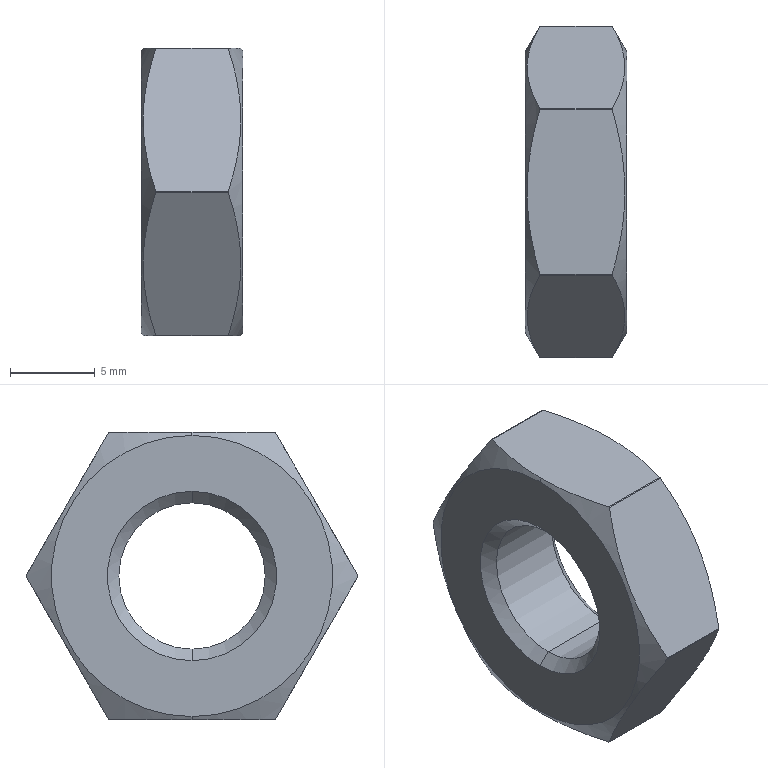Part | STEP file | Guide wheel mechanism revised.sldasm-Part-471 | 1 solid | 24 faces | box 6 x 19.6 x 17 mm | volume 1119 mm3 | cone 8 | cylinder 8 | plane 8 | commonest cylinder face diameters 19.6 x6 8.647 x2
STEP:
#1=CARTESIAN_POINT('',(5.324,0.,-4.324));
#2=VERTEX_POINT('',#1);
#3=CARTESIAN_POINT('',(5.324,0.,4.324));
#4=VERTEX_POINT('',#3);
#5=CARTESIAN_POINT('',(5.324,0.,0.));
#6=DIRECTION('',(-1.,0.,0.));
#7=DIRECTION('',(0.,0.,1.));
#8=AXIS2_PLACEMENT_3D('',#5,#6,#7);
#9=CIRCLE('',#8,4.324);
#10=EDGE_CURVE('',#2,#4,#9,.T.);
#11=ORIENTED_EDGE('',*,*,#10,.T.);
#12=CARTESIAN_POINT('',(6.,0.,5.));
#13=VERTEX_POINT('',#12);
#14=CARTESIAN_POINT('',(6.,0.,5.));
#15=DIRECTION('',(0.7071,0.,0.7071));
#16=VECTOR('',#15,1000.);
#17=LINE('',#14,#16);
#18=EDGE_CURVE('',#4,#13,#17,.T.);
#19=ORIENTED_EDGE('',*,*,#18,.T.);
#20=CARTESIAN_POINT('',(6.,0.,-5.));
#21=VERTEX_POINT('',#20);
#22=CARTESIAN_POINT('',(6.,0.,0.));
#23=DIRECTION('',(-1.,0.,0.));
#24=DIRECTION('',(0.,0.,1.));
#25=AXIS2_PLACEMENT_3D('',#22,#23,#24);
#26=CIRCLE('',#25,5.);
#27=EDGE_CURVE('',#21,#13,#26,.T.);
#28=ORIENTED_EDGE('',*,*,#27,.F.);
#29=CARTESIAN_POINT('',(6.,0.,-5.));
#30=DIRECTION('',(0.7071,0.,-0.7071));
#31=VECTOR('',#30,1000.);
#32=LINE('',#29,#31);
#33=EDGE_CURVE('',#2,#21,#32,.T.);
#34=ORIENTED_EDGE('',*,*,#33,.F.);
#35=EDGE_LOOP('',(#11,#19,#28,#34));
#36=FACE_OUTER_BOUND('',#35,.T.);
#37=CARTESIAN_POINT('',(6.,0.,0.));
#38=DIRECTION('',(1.,0.,0.));
#39=DIRECTION('',(0.,0.,-1.));
#40=AXIS2_PLACEMENT_3D('',#37,#38,#39);
#41=CONICAL_SURFACE('',#40,5.,0.7854);
#42=ADVANCED_FACE('',(#36),#41,.F.);
#43=ORIENTED_EDGE('',*,*,#10,.F.);
#44=CARTESIAN_POINT('',(0.6765,0.,-4.324));
#45=VERTEX_POINT('',#44);
#46=CARTESIAN_POINT('',(6.,0.,-4.324));
#47=DIRECTION('',(-1.,0.,0.));
#48=VECTOR('',#47,1000.);
#49=LINE('',#46,#48);
#50=EDGE_CURVE('',#2,#45,#49,.T.);
#51=ORIENTED_EDGE('',*,*,#50,.T.);
#52=CARTESIAN_POINT('',(0.6765,0.,4.324));
#53=VERTEX_POINT('',#52);
#54=CARTESIAN_POINT('',(0.6765,0.,0.));
#55=DIRECTION('',(-1.,0.,0.));
#56=DIRECTION('',(0.,0.,1.));
#57=AXIS2_PLACEMENT_3D('',#54,#55,#56);
#58=CIRCLE('',#57,4.324);
#59=EDGE_CURVE('',#45,#53,#58,.T.);
#60=ORIENTED_EDGE('',*,*,#59,.T.);
#61=CARTESIAN_POINT('',(6.,0.,4.324));
#62=DIRECTION('',(-1.,0.,0.));
#63=VECTOR('',#62,1000.);
#64=LINE('',#61,#63);
#65=EDGE_CURVE('',#4,#53,#64,.T.);
#66=ORIENTED_EDGE('',*,*,#65,.F.);
#67=EDGE_LOOP('',(#43,#51,#60,#66));
#68=FACE_OUTER_BOUND('',#67,.T.);
#69=CARTESIAN_POINT('',(6.,0.,0.));
#70=DIRECTION('',(-1.,0.,0.));
#71=DIRECTION('',(0.,0.,1.));
#72=AXIS2_PLACEMENT_3D('',#69,#70,#71);
#73=CYLINDRICAL_SURFACE('',#72,4.324);
#74=ADVANCED_FACE('',(#68),#73,.F.);
#75=ORIENTED_EDGE('',*,*,#59,.F.);
#76=CARTESIAN_POINT('',(0.,0.,-5.));
#77=VERTEX_POINT('',#76);
#78=CARTESIAN_POINT('',(0.6765,0.,-4.324));
#79=DIRECTION('',(-0.7071,0.,-0.7071));
#80=VECTOR('',#79,1000.);
#81=LINE('',#78,#80);
#82=EDGE_CURVE('',#45,#77,#81,.T.);
#83=ORIENTED_EDGE('',*,*,#82,.T.);
#84=CARTESIAN_POINT('',(0.,0.,5.));
#85=VERTEX_POINT('',#84);
#86=CARTESIAN_POINT('',(0.,0.,0.));
#87=DIRECTION('',(-1.,0.,0.));
#88=DIRECTION('',(0.,0.,1.));
#89=AXIS2_PLACEMENT_3D('',#86,#87,#88);
#90=CIRCLE('',#89,5.);
#91=EDGE_CURVE('',#77,#85,#90,.T.);
#92=ORIENTED_EDGE('',*,*,#91,.T.);
#93=CARTESIAN_POINT('',(0.6765,0.,4.324));
#94=DIRECTION('',(-0.7071,0.,0.7071));
#95=VECTOR('',#94,1000.);
#96=LINE('',#93,#95);
#97=EDGE_CURVE('',#53,#85,#96,.T.);
#98=ORIENTED_EDGE('',*,*,#97,.F.);
#99=EDGE_LOOP('',(#75,#83,#92,#98));
#100=FACE_OUTER_BOUND('',#99,.T.);
#101=CARTESIAN_POINT('',(0.6765,0.,0.));
#102=DIRECTION('',(-1.,0.,0.));
#103=DIRECTION('',(0.,0.,1.));
#104=AXIS2_PLACEMENT_3D('',#101,#102,#103);
#105=CONICAL_SURFACE('',#104,4.324,0.7854);
#106=ADVANCED_FACE('',(#100),#105,.F.);
#107=CARTESIAN_POINT('',(6.,0.,8.3));
#108=VERTEX_POINT('',#107);
#109=CARTESIAN_POINT('',(6.,0.,-8.3));
#110=VERTEX_POINT('',#109);
#111=CARTESIAN_POINT('',(6.,0.,0.));
#112=DIRECTION('',(-1.,0.,0.));
#113=DIRECTION('',(0.,0.,1.));
#114=AXIS2_PLACEMENT_3D('',#111,#112,#113);
#115=CIRCLE('',#114,8.3);
#116=EDGE_CURVE('',#108,#110,#115,.T.);
#117=ORIENTED_EDGE('',*,*,#116,.T.);
#118=CARTESIAN_POINT('',(5.885,0.,-8.5));
#119=VERTEX_POINT('',#118);
#120=CARTESIAN_POINT('',(6.,0.,-8.3));
#121=DIRECTION('',(-0.5,0.,-0.866));
#122=VECTOR('',#121,1000.);
#123=LINE('',#120,#122);
#124=EDGE_CURVE('',#110,#119,#123,.T.);
#125=ORIENTED_EDGE('',*,*,#124,.T.);
#126=CARTESIAN_POINT('',(5.134,4.877,-8.5));
#127=VERTEX_POINT('',#126);
#128=CARTESIAN_POINT('',(5.885,0.,-8.5));
#129=CARTESIAN_POINT('',(5.885,0.8245,-8.5));
#130=CARTESIAN_POINT('',(5.812,1.66,-8.5));
#131=CARTESIAN_POINT('',(5.549,3.29,-8.5));
#132=CARTESIAN_POINT('',(5.361,4.089,-8.5));
#133=CARTESIAN_POINT('',(5.134,4.877,-8.5));
#134=B_SPLINE_CURVE_WITH_KNOTS('',3,(#128,#129,#130,#131,#132,#133),.UNSPECIFIED.,.F.,.F.,(4,2,4),(0.0137,0.01617,0.01864),.UNSPECIFIED.);
#135=EDGE_CURVE('',#119,#127,#134,.T.);
#136=ORIENTED_EDGE('',*,*,#135,.T.);
#137=CARTESIAN_POINT('',(5.134,4.922,-8.474));
#138=VERTEX_POINT('',#137);
#139=CARTESIAN_POINT('',(5.134,0.,0.));
#140=DIRECTION('',(-1.,0.,0.));
#141=DIRECTION('',(0.,0.,1.));
#142=AXIS2_PLACEMENT_3D('',#139,#140,#141);
#143=CIRCLE('',#142,9.8);
#144=EDGE_CURVE('',#138,#127,#143,.T.);
#145=ORIENTED_EDGE('',*,*,#144,.F.);
#146=CARTESIAN_POINT('',(5.134,9.8,-0.02596));
#147=VERTEX_POINT('',#146);
#148=CARTESIAN_POINT('',(5.134,4.922,-8.474));
#149=CARTESIAN_POINT('',(5.363,5.321,-7.784));
#150=CARTESIAN_POINT('',(5.551,5.722,-7.089));
#151=CARTESIAN_POINT('',(5.812,6.532,-5.686));
#152=CARTESIAN_POINT('',(5.884,6.942,-4.976));
#153=CARTESIAN_POINT('',(5.885,7.564,-3.9));
#154=CARTESIAN_POINT('',(5.867,7.772,-3.539));
#155=CARTESIAN_POINT('',(5.799,8.184,-2.825));
#156=CARTESIAN_POINT('',(5.748,8.389,-2.47));
#157=CARTESIAN_POINT('',(5.552,8.999,-1.413));
#158=CARTESIAN_POINT('',(5.363,9.401,-0.7167));
#159=CARTESIAN_POINT('',(5.134,9.8,-0.02596));
#160=B_SPLINE_CURVE_WITH_KNOTS('',3,(#148,#149,#150,#151,#152,#153,#154,#155,#156,#157,#158,#159),.UNSPECIFIED.,.F.,.F.,(4,2,2,2,2,4),(0.000000717,0.002463,0.004926,0.006157,0.007388,0.00985),.UNSPECIFIED.);
#161=EDGE_CURVE('',#138,#147,#160,.T.);
#162=ORIENTED_EDGE('',*,*,#161,.T.);
#163=CARTESIAN_POINT('',(5.134,9.8,0.02596));
#164=VERTEX_POINT('',#163);
#165=CARTESIAN_POINT('',(5.134,0.,0.));
#166=DIRECTION('',(-1.,0.,0.));
#167=DIRECTION('',(0.,0.,1.));
#168=AXIS2_PLACEMENT_3D('',#165,#166,#167);
#169=CIRCLE('',#168,9.8);
#170=EDGE_CURVE('',#164,#147,#169,.T.);
#171=ORIENTED_EDGE('',*,*,#170,.F.);
#172=CARTESIAN_POINT('',(5.134,4.922,8.474));
#173=VERTEX_POINT('',#172);
#174=CARTESIAN_POINT('',(5.134,9.8,0.02596));
#175=CARTESIAN_POINT('',(5.363,9.402,0.7158));
#176=CARTESIAN_POINT('',(5.551,9.001,1.411));
#177=CARTESIAN_POINT('',(5.812,8.19,2.814));
#178=CARTESIAN_POINT('',(5.884,7.781,3.524));
#179=CARTESIAN_POINT('',(5.885,7.159,4.6));
#180=CARTESIAN_POINT('',(5.867,6.951,4.961));
#181=CARTESIAN_POINT('',(5.799,6.538,5.675));
#182=CARTESIAN_POINT('',(5.748,6.334,6.03));
#183=CARTESIAN_POINT('',(5.552,5.723,7.087));
#184=CARTESIAN_POINT('',(5.363,5.321,7.783));
#185=CARTESIAN_POINT('',(5.134,4.922,8.474));
#186=B_SPLINE_CURVE_WITH_KNOTS('',3,(#174,#175,#176,#177,#178,#179,#180,#181,#182,#183,#184,#185),.UNSPECIFIED.,.F.,.F.,(4,2,2,2,2,4),(0.000000483,0.002463,0.004925,0.006157,0.007388,0.00985),.UNSPECIFIED.);
#187=EDGE_CURVE('',#164,#173,#186,.T.);
#188=ORIENTED_EDGE('',*,*,#187,.T.);
#189=CARTESIAN_POINT('',(5.134,4.877,8.5));
#190=VERTEX_POINT('',#189);
#191=CARTESIAN_POINT('',(5.134,0.,0.));
#192=DIRECTION('',(-1.,0.,0.));
#193=DIRECTION('',(0.,0.,1.));
#194=AXIS2_PLACEMENT_3D('',#191,#192,#193);
#195=CIRCLE('',#194,9.8);
#196=EDGE_CURVE('',#190,#173,#195,.T.);
#197=ORIENTED_EDGE('',*,*,#196,.F.);
#198=CARTESIAN_POINT('',(5.885,0.,8.5));
#199=VERTEX_POINT('',#198);
#200=CARTESIAN_POINT('',(5.134,4.877,8.5));
#201=CARTESIAN_POINT('',(5.361,4.089,8.5));
#202=CARTESIAN_POINT('',(5.549,3.29,8.5));
#203=CARTESIAN_POINT('',(5.812,1.66,8.5));
#204=CARTESIAN_POINT('',(5.885,0.8245,8.5));
#205=CARTESIAN_POINT('',(5.885,0.,8.5));
#206=B_SPLINE_CURVE_WITH_KNOTS('',3,(#200,#201,#202,#203,#204,#205),.UNSPECIFIED.,.F.,.F.,(4,2,4),(0.003649,0.006111,0.008573),.UNSPECIFIED.);
#207=EDGE_CURVE('',#190,#199,#206,.T.);
#208=ORIENTED_EDGE('',*,*,#207,.T.);
#209=CARTESIAN_POINT('',(6.,0.,8.3));
#210=DIRECTION('',(-0.5,0.,0.866));
#211=VECTOR('',#210,1000.);
#212=LINE('',#209,#211);
#213=EDGE_CURVE('',#108,#199,#212,.T.);
#214=ORIENTED_EDGE('',*,*,#213,.F.);
#215=EDGE_LOOP('',(#117,#125,#136,#145,#162,#171,#188,#197,#208,#214));
#216=FACE_OUTER_BOUND('',#215,.T.);
#217=CARTESIAN_POINT('',(6.,0.,0.));
#218=DIRECTION('',(-1.,0.,0.));
#219=DIRECTION('',(0.,0.,1.));
#220=AXIS2_PLACEMENT_3D('',#217,#218,#219);
#221=CONICAL_SURFACE('',#220,8.3,1.047);
#222=ADVANCED_FACE('',(#216),#221,.T.);
#223=CARTESIAN_POINT('',(0.,0.,8.3));
#224=VERTEX_POINT('',#223);
#225=CARTESIAN_POINT('',(0.,0.,-8.3));
#226=VERTEX_POINT('',#225);
#227=CARTESIAN_POINT('',(0.,0.,0.));
#228=DIRECTION('',(-1.,0.,0.));
#229=DIRECTION('',(0.,0.,1.));
#230=AXIS2_PLACEMENT_3D('',#227,#228,#229);
#231=CIRCLE('',#230,8.3);
#232=EDGE_CURVE('',#224,#226,#231,.T.);
#233=ORIENTED_EDGE('',*,*,#232,.F.);
#234=CARTESIAN_POINT('',(0.1155,0.,8.5));
#235=VERTEX_POINT('',#234);
#236=CARTESIAN_POINT('',(0.866,0.,9.8));
#237=DIRECTION('',(0.5,0.,0.866));
#238=VECTOR('',#237,1000.);
#239=LINE('',#236,#238);
#240=EDGE_CURVE('',#224,#235,#239,.T.);
#241=ORIENTED_EDGE('',*,*,#240,.T.);
#242=CARTESIAN_POINT('',(0.866,4.877,8.5));
#243=VERTEX_POINT('',#242);
#244=CARTESIAN_POINT('',(0.1155,0.,8.5));
#245=CARTESIAN_POINT('',(0.1155,0.8245,8.5));
#246=CARTESIAN_POINT('',(0.1878,1.66,8.5));
#247=CARTESIAN_POINT('',(0.4508,3.29,8.5));
#248=CARTESIAN_POINT('',(0.6394,4.089,8.5));
#249=CARTESIAN_POINT('',(0.866,4.877,8.5));
#250=B_SPLINE_CURVE_WITH_KNOTS('',3,(#244,#245,#246,#247,#248,#249),.UNSPECIFIED.,.F.,.F.,(4,2,4),(0.0137,0.01617,0.01864),.UNSPECIFIED.);
#251=EDGE_CURVE('',#235,#243,#250,.T.);
#252=ORIENTED_EDGE('',*,*,#251,.T.);
#253=CARTESIAN_POINT('',(0.866,4.922,8.474));
#254=VERTEX_POINT('',#253);
#255=CARTESIAN_POINT('',(0.866,0.,0.));
#256=DIRECTION('',(-1.,0.,0.));
#257=DIRECTION('',(0.,0.,1.));
#258=AXIS2_PLACEMENT_3D('',#255,#256,#257);
#259=CIRCLE('',#258,9.8);
#260=EDGE_CURVE('',#243,#254,#259,.T.);
#261=ORIENTED_EDGE('',*,*,#260,.T.);
#262=CARTESIAN_POINT('',(0.866,9.8,0.02596));
#263=VERTEX_POINT('',#262);
#264=CARTESIAN_POINT('',(0.866,4.922,8.474));
#265=CARTESIAN_POINT('',(0.6371,5.321,7.784));
#266=CARTESIAN_POINT('',(0.4487,5.722,7.089));
#267=CARTESIAN_POINT('',(0.1877,6.532,5.686));
#268=CARTESIAN_POINT('',(0.116,6.942,4.976));
#269=CARTESIAN_POINT('',(0.1152,7.564,3.9));
#270=CARTESIAN_POINT('',(0.1327,7.772,3.539));
#271=CARTESIAN_POINT('',(0.201,8.184,2.825));
#272=CARTESIAN_POINT('',(0.2518,8.389,2.47));
#273=CARTESIAN_POINT('',(0.4479,8.999,1.413));
#274=CARTESIAN_POINT('',(0.6368,9.401,0.7167));
#275=CARTESIAN_POINT('',(0.866,9.8,0.02596));
#276=B_SPLINE_CURVE_WITH_KNOTS('',3,(#264,#265,#266,#267,#268,#269,#270,#271,#272,#273,#274,#275),.UNSPECIFIED.,.F.,.F.,(4,2,2,2,2,4),(0.000000717,0.002463,0.004926,0.006157,0.007388,0.00985),.UNSPECIFIED.);
#277=EDGE_CURVE('',#254,#263,#276,.T.);
#278=ORIENTED_EDGE('',*,*,#277,.T.);
#279=CARTESIAN_POINT('',(0.866,9.8,-0.02596));
#280=VERTEX_POINT('',#279);
#281=CARTESIAN_POINT('',(0.866,0.,0.));
#282=DIRECTION('',(-1.,0.,0.));
#283=DIRECTION('',(0.,0.,1.));
#284=AXIS2_PLACEMENT_3D('',#281,#282,#283);
#285=CIRCLE('',#284,9.8);
#286=EDGE_CURVE('',#263,#280,#285,.T.);
#287=ORIENTED_EDGE('',*,*,#286,.T.);
#288=CARTESIAN_POINT('',(0.866,4.922,-8.474));
#289=VERTEX_POINT('',#288);
#290=CARTESIAN_POINT('',(0.866,9.8,-0.02596));
#291=CARTESIAN_POINT('',(0.6371,9.402,-0.7158));
#292=CARTESIAN_POINT('',(0.4487,9.001,-1.411));
#293=CARTESIAN_POINT('',(0.1877,8.19,-2.814));
#294=CARTESIAN_POINT('',(0.116,7.781,-3.524));
#295=CARTESIAN_POINT('',(0.1152,7.159,-4.6));
#296=CARTESIAN_POINT('',(0.1327,6.951,-4.961));
#297=CARTESIAN_POINT('',(0.201,6.538,-5.675));
#298=CARTESIAN_POINT('',(0.2518,6.334,-6.03));
#299=CARTESIAN_POINT('',(0.4479,5.723,-7.087));
#300=CARTESIAN_POINT('',(0.6368,5.321,-7.783));
#301=CARTESIAN_POINT('',(0.866,4.922,-8.474));
#302=B_SPLINE_CURVE_WITH_KNOTS('',3,(#290,#291,#292,#293,#294,#295,#296,#297,#298,#299,#300,#301),.UNSPECIFIED.,.F.,.F.,(4,2,2,2,2,4),(0.000000483,0.002463,0.004925,0.006157,0.007388,0.00985),.UNSPECIFIED.);
#303=EDGE_CURVE('',#280,#289,#302,.T.);
#304=ORIENTED_EDGE('',*,*,#303,.T.);
#305=CARTESIAN_POINT('',(0.866,4.877,-8.5));
#306=VERTEX_POINT('',#305);
#307=CARTESIAN_POINT('',(0.866,0.,0.));
#308=DIRECTION('',(-1.,0.,0.));
#309=DIRECTION('',(0.,0.,1.));
#310=AXIS2_PLACEMENT_3D('',#307,#308,#309);
#311=CIRCLE('',#310,9.8);
#312=EDGE_CURVE('',#289,#306,#311,.T.);
#313=ORIENTED_EDGE('',*,*,#312,.T.);
#314=CARTESIAN_POINT('',(0.1155,0.,-8.5));
#315=VERTEX_POINT('',#314);
#316=CARTESIAN_POINT('',(0.866,4.877,-8.5));
#317=CARTESIAN_POINT('',(0.6394,4.089,-8.5));
#318=CARTESIAN_POINT('',(0.4508,3.29,-8.5));
#319=CARTESIAN_POINT('',(0.1878,1.66,-8.5));
#320=CARTESIAN_POINT('',(0.1155,0.8245,-8.5));
#321=CARTESIAN_POINT('',(0.1155,0.,-8.5));
#322=B_SPLINE_CURVE_WITH_KNOTS('',3,(#316,#317,#318,#319,#320,#321),.UNSPECIFIED.,.F.,.F.,(4,2,4),(0.003649,0.006111,0.008573),.UNSPECIFIED.);
#323=EDGE_CURVE('',#306,#315,#322,.T.);
#324=ORIENTED_EDGE('',*,*,#323,.T.);
#325=CARTESIAN_POINT('',(0.866,0.,-9.8));
#326=DIRECTION('',(0.5,0.,-0.866));
#327=VECTOR('',#326,1000.);
#328=LINE('',#325,#327);
#329=EDGE_CURVE('',#226,#315,#328,.T.);
#330=ORIENTED_EDGE('',*,*,#329,.F.);
#331=EDGE_LOOP('',(#233,#241,#252,#261,#278,#287,#304,#313,#324,#330));
#332=FACE_OUTER_BOUND('',#331,.T.);
#333=CARTESIAN_POINT('',(0.866,0.,0.));
#334=DIRECTION('',(1.,0.,0.));
#335=DIRECTION('',(0.,0.,-1.));
#336=AXIS2_PLACEMENT_3D('',#333,#334,#335);
#337=CONICAL_SURFACE('',#336,9.8,1.047);
#338=ADVANCED_FACE('',(#332),#337,.T.);
#339=CARTESIAN_POINT('',(0.,0.,0.));
#340=DIRECTION('',(-1.,0.,0.));
#341=DIRECTION('',(0.,0.,1.));
#342=AXIS2_PLACEMENT_3D('',#339,#340,#341);
#343=CIRCLE('',#342,8.3);
#344=EDGE_CURVE('',#226,#224,#343,.T.);
#345=ORIENTED_EDGE('',*,*,#344,.T.);
#346=ORIENTED_EDGE('',*,*,#232,.T.);
#347=EDGE_LOOP('',(#345,#346));
#348=FACE_OUTER_BOUND('',#347,.T.);
#349=CARTESIAN_POINT('',(0.,0.,0.));
#350=DIRECTION('',(-1.,0.,0.));
#351=DIRECTION('',(0.,0.,1.));
#352=AXIS2_PLACEMENT_3D('',#349,#350,#351);
#353=CIRCLE('',#352,5.);
#354=EDGE_CURVE('',#85,#77,#353,.T.);
#355=ORIENTED_EDGE('',*,*,#354,.F.);
#356=ORIENTED_EDGE('',*,*,#91,.F.);
#357=EDGE_LOOP('',(#355,#356));
#358=FACE_BOUND('',#357,.T.);
#359=CARTESIAN_POINT('',(0.,0.,0.));
#360=DIRECTION('',(1.,0.,0.));
#361=DIRECTION('',(0.,0.,-1.));
#362=AXIS2_PLACEMENT_3D('',#359,#360,#361);
#363=PLANE('',#362);
#364=ADVANCED_FACE('',(#348,#358),#363,.F.);
#365=ORIENTED_EDGE('',*,*,#116,.F.);
#366=CARTESIAN_POINT('',(6.,0.,0.));
#367=DIRECTION('',(-1.,0.,0.));
#368=DIRECTION('',(0.,0.,1.));
#369=AXIS2_PLACEMENT_3D('',#366,#367,#368);
#370=CIRCLE('',#369,8.3);
#371=EDGE_CURVE('',#110,#108,#370,.T.);
#372=ORIENTED_EDGE('',*,*,#371,.F.);
#373=EDGE_LOOP('',(#365,#372));
#374=FACE_OUTER_BOUND('',#373,.T.);
#375=ORIENTED_EDGE('',*,*,#27,.T.);
#376=CARTESIAN_POINT('',(6.,0.,0.));
#377=DIRECTION('',(-1.,0.,0.));
#378=DIRECTION('',(0.,0.,1.));
#379=AXIS2_PLACEMENT_3D('',#376,#377,#378);
#380=CIRCLE('',#379,5.);
#381=EDGE_CURVE('',#13,#21,#380,.T.);
#382=ORIENTED_EDGE('',*,*,#381,.T.);
#383=EDGE_LOOP('',(#375,#382));
#384=FACE_BOUND('',#383,.T.);
#385=CARTESIAN_POINT('',(6.,8.3,0.));
#386=DIRECTION('',(-1.,0.,0.));
#387=DIRECTION('',(0.,0.,1.));
#388=AXIS2_PLACEMENT_3D('',#385,#386,#387);
#389=PLANE('',#388);
#390=ADVANCED_FACE('',(#374,#384),#389,.F.);
#391=ORIENTED_EDGE('',*,*,#196,.T.);
#392=CARTESIAN_POINT('',(6.,4.922,8.474));
#393=DIRECTION('',(-1.,0.,0.));
#394=VECTOR('',#393,1000.);
#395=LINE('',#392,#394);
#396=EDGE_CURVE('',#173,#254,#395,.T.);
#397=ORIENTED_EDGE('',*,*,#396,.T.);
#398=ORIENTED_EDGE('',*,*,#260,.F.);
#399=CARTESIAN_POINT('',(6.,4.877,8.5));
#400=DIRECTION('',(1.,0.,0.));
#401=VECTOR('',#400,1000.);
#402=LINE('',#399,#401);
#403=EDGE_CURVE('',#243,#190,#402,.T.);
#404=ORIENTED_EDGE('',*,*,#403,.T.);
#405=EDGE_LOOP('',(#391,#397,#398,#404));
#406=FACE_OUTER_BOUND('',#405,.T.);
#407=CARTESIAN_POINT('',(6.,0.,0.));
#408=DIRECTION('',(-1.,0.,0.));
#409=DIRECTION('',(0.,0.,1.));
#410=AXIS2_PLACEMENT_3D('',#407,#408,#409);
#411=CYLINDRICAL_SURFACE('',#410,9.8);
#412=ADVANCED_FACE('',(#406),#411,.T.);
#413=CARTESIAN_POINT('',(5.134,-4.922,8.474));
#414=VERTEX_POINT('',#413);
#415=CARTESIAN_POINT('',(5.134,-4.877,8.5));
#416=VERTEX_POINT('',#415);
#417=CARTESIAN_POINT('',(5.134,0.,0.));
#418=DIRECTION('',(-1.,0.,0.));
#419=DIRECTION('',(0.,0.,1.));
#420=AXIS2_PLACEMENT_3D('',#417,#418,#419);
#421=CIRCLE('',#420,9.8);
#422=EDGE_CURVE('',#414,#416,#421,.T.);
#423=ORIENTED_EDGE('',*,*,#422,.T.);
#424=CARTESIAN_POINT('',(0.866,-4.877,8.5));
#425=VERTEX_POINT('',#424);
#426=CARTESIAN_POINT('',(6.,-4.877,8.5));
#427=DIRECTION('',(-1.,0.,0.));
#428=VECTOR('',#427,1000.);
#429=LINE('',#426,#428);
#430=EDGE_CURVE('',#416,#425,#429,.T.);
#431=ORIENTED_EDGE('',*,*,#430,.T.);
#432=CARTESIAN_POINT('',(0.866,-4.922,8.474));
#433=VERTEX_POINT('',#432);
#434=CARTESIAN_POINT('',(0.866,0.,0.));
#435=DIRECTION('',(-1.,0.,0.));
#436=DIRECTION('',(0.,0.,1.));
#437=AXIS2_PLACEMENT_3D('',#434,#435,#436);
#438=CIRCLE('',#437,9.8);
#439=EDGE_CURVE('',#433,#425,#438,.T.);
#440=ORIENTED_EDGE('',*,*,#439,.F.);
#441=CARTESIAN_POINT('',(6.,-4.922,8.474));
#442=DIRECTION('',(1.,0.,0.));
#443=VECTOR('',#442,1000.);
#444=LINE('',#441,#443);
#445=EDGE_CURVE('',#433,#414,#444,.T.);
#446=ORIENTED_EDGE('',*,*,#445,.T.);
#447=EDGE_LOOP('',(#423,#431,#440,#446));
#448=FACE_OUTER_BOUND('',#447,.T.);
#449=CARTESIAN_POINT('',(6.,0.,0.));
#450=DIRECTION('',(-1.,0.,0.));
#451=DIRECTION('',(0.,0.,1.));
#452=AXIS2_PLACEMENT_3D('',#449,#450,#451);
#453=CYLINDRICAL_SURFACE('',#452,9.8);
#454=ADVANCED_FACE('',(#448),#453,.T.);
#455=CARTESIAN_POINT('',(5.134,-9.8,-0.02596));
#456=VERTEX_POINT('',#455);
#457=CARTESIAN_POINT('',(5.134,-9.8,0.02596));
#458=VERTEX_POINT('',#457);
#459=CARTESIAN_POINT('',(5.134,0.,0.));
#460=DIRECTION('',(-1.,0.,0.));
#461=DIRECTION('',(0.,0.,1.));
#462=AXIS2_PLACEMENT_3D('',#459,#460,#461);
#463=CIRCLE('',#462,9.8);
#464=EDGE_CURVE('',#456,#458,#463,.T.);
#465=ORIENTED_EDGE('',*,*,#464,.T.);
#466=CARTESIAN_POINT('',(0.866,-9.8,0.02596));
#467=VERTEX_POINT('',#466);
#468=CARTESIAN_POINT('',(6.,-9.8,0.02596));
#469=DIRECTION('',(-1.,0.,0.));
#470=VECTOR('',#469,1000.);
#471=LINE('',#468,#470);
#472=EDGE_CURVE('',#458,#467,#471,.T.);
#473=ORIENTED_EDGE('',*,*,#472,.T.);
#474=CARTESIAN_POINT('',(0.866,-9.8,-0.02596));
#475=VERTEX_POINT('',#474);
#476=CARTESIAN_POINT('',(0.866,0.,0.));
#477=DIRECTION('',(-1.,0.,0.));
#478=DIRECTION('',(0.,0.,1.));
#479=AXIS2_PLACEMENT_3D('',#476,#477,#478);
#480=CIRCLE('',#479,9.8);
#481=EDGE_CURVE('',#475,#467,#480,.T.);
#482=ORIENTED_EDGE('',*,*,#481,.F.);
#483=CARTESIAN_POINT('',(6.,-9.8,-0.02596));
#484=DIRECTION('',(1.,0.,0.));
#485=VECTOR('',#484,1000.);
#486=LINE('',#483,#485);
#487=EDGE_CURVE('',#475,#456,#486,.T.);
#488=ORIENTED_EDGE('',*,*,#487,.T.);
#489=EDGE_LOOP('',(#465,#473,#482,#488));
#490=FACE_OUTER_BOUND('',#489,.T.);
#491=CARTESIAN_POINT('',(6.,0.,0.));
#492=DIRECTION('',(-1.,0.,0.));
#493=DIRECTION('',(0.,0.,1.));
#494=AXIS2_PLACEMENT_3D('',#491,#492,#493);
#495=CYLINDRICAL_SURFACE('',#494,9.8);
#496=ADVANCED_FACE('',(#490),#495,.T.);
#497=CARTESIAN_POINT('',(5.134,-4.877,-8.5));
#498=VERTEX_POINT('',#497);
#499=CARTESIAN_POINT('',(5.134,-4.922,-8.474));
#500=VERTEX_POINT('',#499);
#501=CARTESIAN_POINT('',(5.134,0.,0.));
#502=DIRECTION('',(-1.,0.,0.));
#503=DIRECTION('',(0.,0.,1.));
#504=AXIS2_PLACEMENT_3D('',#501,#502,#503);
#505=CIRCLE('',#504,9.8);
#506=EDGE_CURVE('',#498,#500,#505,.T.);
#507=ORIENTED_EDGE('',*,*,#506,.T.);
#508=CARTESIAN_POINT('',(0.866,-4.922,-8.474));
#509=VERTEX_POINT('',#508);
#510=CARTESIAN_POINT('',(6.,-4.922,-8.474));
#511=DIRECTION('',(-1.,0.,0.));
#512=VECTOR('',#511,1000.);
#513=LINE('',#510,#512);
#514=EDGE_CURVE('',#500,#509,#513,.T.);
#515=ORIENTED_EDGE('',*,*,#514,.T.);
#516=CARTESIAN_POINT('',(0.866,-4.877,-8.5));
#517=VERTEX_POINT('',#516);
#518=CARTESIAN_POINT('',(0.866,0.,0.));
#519=DIRECTION('',(-1.,0.,0.));
#520=DIRECTION('',(0.,0.,1.));
#521=AXIS2_PLACEMENT_3D('',#518,#519,#520);
#522=CIRCLE('',#521,9.8);
#523=EDGE_CURVE('',#517,#509,#522,.T.);
#524=ORIENTED_EDGE('',*,*,#523,.F.);
#525=CARTESIAN_POINT('',(6.,-4.877,-8.5));
#526=DIRECTION('',(1.,0.,0.));
#527=VECTOR('',#526,1000.);
#528=LINE('',#525,#527);
#529=EDGE_CURVE('',#517,#498,#528,.T.);
#530=ORIENTED_EDGE('',*,*,#529,.T.);
#531=EDGE_LOOP('',(#507,#515,#524,#530));
#532=FACE_OUTER_BOUND('',#531,.T.);
#533=CARTESIAN_POINT('',(6.,0.,0.));
#534=DIRECTION('',(-1.,0.,0.));
#535=DIRECTION('',(0.,0.,1.));
#536=AXIS2_PLACEMENT_3D('',#533,#534,#535);
#537=CYLINDRICAL_SURFACE('',#536,9.8);
#538=ADVANCED_FACE('',(#532),#537,.T.);
#539=ORIENTED_EDGE('',*,*,#144,.T.);
#540=CARTESIAN_POINT('',(6.,4.877,-8.5));
#541=DIRECTION('',(-1.,0.,0.));
#542=VECTOR('',#541,1000.);
#543=LINE('',#540,#542);
#544=EDGE_CURVE('',#127,#306,#543,.T.);
#545=ORIENTED_EDGE('',*,*,#544,.T.);
#546=ORIENTED_EDGE('',*,*,#312,.F.);
#547=CARTESIAN_POINT('',(6.,4.922,-8.474));
#548=DIRECTION('',(1.,0.,0.));
#549=VECTOR('',#548,1000.);
#550=LINE('',#547,#549);
#551=EDGE_CURVE('',#289,#138,#550,.T.);
#552=ORIENTED_EDGE('',*,*,#551,.T.);
#553=EDGE_LOOP('',(#539,#545,#546,#552));
#554=FACE_OUTER_BOUND('',#553,.T.);
#555=CARTESIAN_POINT('',(6.,0.,0.));
#556=DIRECTION('',(-1.,0.,0.));
#557=DIRECTION('',(0.,0.,1.));
#558=AXIS2_PLACEMENT_3D('',#555,#556,#557);
#559=CYLINDRICAL_SURFACE('',#558,9.8);
#560=ADVANCED_FACE('',(#554),#559,.T.);
#561=ORIENTED_EDGE('',*,*,#240,.F.);
#562=ORIENTED_EDGE('',*,*,#344,.F.);
#563=ORIENTED_EDGE('',*,*,#329,.T.);
#564=CARTESIAN_POINT('',(0.1155,0.,-8.5));
#565=CARTESIAN_POINT('',(0.1155,-0.824,-8.5));
#566=CARTESIAN_POINT('',(0.1858,-1.643,-8.5));
#567=CARTESIAN_POINT('',(0.447,-3.271,-8.5));
#568=CARTESIAN_POINT('',(0.638,-4.084,-8.5));
#569=CARTESIAN_POINT('',(0.866,-4.877,-8.5));
#570=B_SPLINE_CURVE_WITH_KNOTS('',3,(#564,#565,#566,#567,#568,#569),.UNSPECIFIED.,.F.,.F.,(4,2,4),(0.008573,0.01103,0.01349),.UNSPECIFIED.);
#571=EDGE_CURVE('',#315,#517,#570,.T.);
#572=ORIENTED_EDGE('',*,*,#571,.T.);
#573=ORIENTED_EDGE('',*,*,#523,.T.);
#574=CARTESIAN_POINT('',(0.866,-4.922,-8.474));
#575=CARTESIAN_POINT('',(0.6371,-5.321,-7.784));
#576=CARTESIAN_POINT('',(0.4487,-5.722,-7.089));
#577=CARTESIAN_POINT('',(0.1877,-6.532,-5.686));
#578=CARTESIAN_POINT('',(0.116,-6.942,-4.976));
#579=CARTESIAN_POINT('',(0.1152,-7.564,-3.9));
#580=CARTESIAN_POINT('',(0.1327,-7.772,-3.539));
#581=CARTESIAN_POINT('',(0.201,-8.184,-2.825));
#582=CARTESIAN_POINT('',(0.2518,-8.389,-2.47));
#583=CARTESIAN_POINT('',(0.4479,-8.999,-1.413));
#584=CARTESIAN_POINT('',(0.6368,-9.401,-0.7167));
#585=CARTESIAN_POINT('',(0.866,-9.8,-0.02596));
#586=B_SPLINE_CURVE_WITH_KNOTS('',3,(#574,#575,#576,#577,#578,#579,#580,#581,#582,#583,#584,#585),.UNSPECIFIED.,.F.,.F.,(4,2,2,2,2,4),(0.000000717,0.002463,0.004926,0.006157,0.007388,0.00985),.UNSPECIFIED.);
#587=EDGE_CURVE('',#509,#475,#586,.T.);
#588=ORIENTED_EDGE('',*,*,#587,.T.);
#589=ORIENTED_EDGE('',*,*,#481,.T.);
#590=CARTESIAN_POINT('',(0.866,-9.8,0.02596));
#591=CARTESIAN_POINT('',(0.6371,-9.402,0.7158));
#592=CARTESIAN_POINT('',(0.4487,-9.001,1.411));
#593=CARTESIAN_POINT('',(0.1877,-8.19,2.814));
#594=CARTESIAN_POINT('',(0.116,-7.781,3.524));
#595=CARTESIAN_POINT('',(0.1152,-7.159,4.6));
#596=CARTESIAN_POINT('',(0.1327,-6.951,4.961));
#597=CARTESIAN_POINT('',(0.201,-6.538,5.675));
#598=CARTESIAN_POINT('',(0.2518,-6.334,6.03));
#599=CARTESIAN_POINT('',(0.4479,-5.723,7.087));
#600=CARTESIAN_POINT('',(0.6368,-5.321,7.783));
#601=CARTESIAN_POINT('',(0.866,-4.922,8.474));
#602=B_SPLINE_CURVE_WITH_KNOTS('',3,(#590,#591,#592,#593,#594,#595,#596,#597,#598,#599,#600,#601),.UNSPECIFIED.,.F.,.F.,(4,2,2,2,2,4),(0.000000483,0.002463,0.004925,0.006157,0.007388,0.00985),.UNSPECIFIED.);
#603=EDGE_CURVE('',#467,#433,#602,.T.);
#604=ORIENTED_EDGE('',*,*,#603,.T.);
#605=ORIENTED_EDGE('',*,*,#439,.T.);
#606=CARTESIAN_POINT('',(0.866,-4.877,8.5));
#607=CARTESIAN_POINT('',(0.638,-4.084,8.5));
#608=CARTESIAN_POINT('',(0.447,-3.271,8.5));
#609=CARTESIAN_POINT('',(0.1858,-1.643,8.5));
#610=CARTESIAN_POINT('',(0.1155,-0.824,8.5));
#611=CARTESIAN_POINT('',(0.1155,0.,8.5));
#612=B_SPLINE_CURVE_WITH_KNOTS('',3,(#606,#607,#608,#609,#610,#611),.UNSPECIFIED.,.F.,.F.,(4,2,4),(0.008768,0.01123,0.0137),.UNSPECIFIED.);
#613=EDGE_CURVE('',#425,#235,#612,.T.);
#614=ORIENTED_EDGE('',*,*,#613,.T.);
#615=EDGE_LOOP('',(#561,#562,#563,#572,#573,#588,#589,#604,#605,#614));
#616=FACE_OUTER_BOUND('',#615,.T.);
#617=CARTESIAN_POINT('',(0.866,0.,0.));
#618=DIRECTION('',(1.,0.,0.));
#619=DIRECTION('',(0.,0.,-1.));
#620=AXIS2_PLACEMENT_3D('',#617,#618,#619);
#621=CONICAL_SURFACE('',#620,9.8,1.047);
#622=ADVANCED_FACE('',(#616),#621,.T.);
#623=ORIENTED_EDGE('',*,*,#286,.F.);
#624=CARTESIAN_POINT('',(6.,9.8,0.02596));
#625=DIRECTION('',(1.,0.,0.));
#626=VECTOR('',#625,1000.);
#627=LINE('',#624,#626);
#628=EDGE_CURVE('',#263,#164,#627,.T.);
#629=ORIENTED_EDGE('',*,*,#628,.T.);
#630=ORIENTED_EDGE('',*,*,#170,.T.);
#631=CARTESIAN_POINT('',(6.,9.8,-0.02596));
#632=DIRECTION('',(-1.,0.,0.));
#633=VECTOR('',#632,1000.);
#634=LINE('',#631,#633);
#635=EDGE_CURVE('',#147,#280,#634,.T.);
#636=ORIENTED_EDGE('',*,*,#635,.T.);
#637=EDGE_LOOP('',(#623,#629,#630,#636));
#638=FACE_OUTER_BOUND('',#637,.T.);
#639=CARTESIAN_POINT('',(6.,0.,0.));
#640=DIRECTION('',(-1.,0.,0.));
#641=DIRECTION('',(0.,0.,1.));
#642=AXIS2_PLACEMENT_3D('',#639,#640,#641);
#643=CYLINDRICAL_SURFACE('',#642,9.8);
#644=ADVANCED_FACE('',(#638),#643,.T.);
#645=ORIENTED_EDGE('',*,*,#124,.F.);
#646=ORIENTED_EDGE('',*,*,#371,.T.);
#647=ORIENTED_EDGE('',*,*,#213,.T.);
#648=CARTESIAN_POINT('',(5.885,0.,8.5));
#649=CARTESIAN_POINT('',(5.885,-0.824,8.5));
#650=CARTESIAN_POINT('',(5.814,-1.643,8.5));
#651=CARTESIAN_POINT('',(5.553,-3.271,8.5));
#652=CARTESIAN_POINT('',(5.362,-4.084,8.5));
#653=CARTESIAN_POINT('',(5.134,-4.877,8.5));
#654=B_SPLINE_CURVE_WITH_KNOTS('',3,(#648,#649,#650,#651,#652,#653),.UNSPECIFIED.,.F.,.F.,(4,2,4),(0.008573,0.01103,0.01349),.UNSPECIFIED.);
#655=EDGE_CURVE('',#199,#416,#654,.T.);
#656=ORIENTED_EDGE('',*,*,#655,.T.);
#657=ORIENTED_EDGE('',*,*,#422,.F.);
#658=CARTESIAN_POINT('',(5.134,-4.922,8.474));
#659=CARTESIAN_POINT('',(5.363,-5.321,7.784));
#660=CARTESIAN_POINT('',(5.551,-5.722,7.089));
#661=CARTESIAN_POINT('',(5.812,-6.532,5.686));
#662=CARTESIAN_POINT('',(5.884,-6.942,4.976));
#663=CARTESIAN_POINT('',(5.885,-7.564,3.9));
#664=CARTESIAN_POINT('',(5.867,-7.772,3.539));
#665=CARTESIAN_POINT('',(5.799,-8.184,2.825));
#666=CARTESIAN_POINT('',(5.748,-8.389,2.47));
#667=CARTESIAN_POINT('',(5.552,-8.999,1.413));
#668=CARTESIAN_POINT('',(5.363,-9.401,0.7167));
#669=CARTESIAN_POINT('',(5.134,-9.8,0.02596));
#670=B_SPLINE_CURVE_WITH_KNOTS('',3,(#658,#659,#660,#661,#662,#663,#664,#665,#666,#667,#668,#669),.UNSPECIFIED.,.F.,.F.,(4,2,2,2,2,4),(0.000000717,0.002463,0.004926,0.006157,0.007388,0.00985),.UNSPECIFIED.);
#671=EDGE_CURVE('',#414,#458,#670,.T.);
#672=ORIENTED_EDGE('',*,*,#671,.T.);
#673=ORIENTED_EDGE('',*,*,#464,.F.);
#674=CARTESIAN_POINT('',(5.134,-9.8,-0.02596));
#675=CARTESIAN_POINT('',(5.363,-9.402,-0.7158));
#676=CARTESIAN_POINT('',(5.551,-9.001,-1.411));
#677=CARTESIAN_POINT('',(5.812,-8.19,-2.814));
#678=CARTESIAN_POINT('',(5.884,-7.781,-3.524));
#679=CARTESIAN_POINT('',(5.885,-7.159,-4.6));
#680=CARTESIAN_POINT('',(5.867,-6.951,-4.961));
#681=CARTESIAN_POINT('',(5.799,-6.538,-5.675));
#682=CARTESIAN_POINT('',(5.748,-6.334,-6.03));
#683=CARTESIAN_POINT('',(5.552,-5.723,-7.087));
#684=CARTESIAN_POINT('',(5.363,-5.321,-7.783));
#685=CARTESIAN_POINT('',(5.134,-4.922,-8.474));
#686=B_SPLINE_CURVE_WITH_KNOTS('',3,(#674,#675,#676,#677,#678,#679,#680,#681,#682,#683,#684,#685),.UNSPECIFIED.,.F.,.F.,(4,2,2,2,2,4),(0.000000483,0.002463,0.004925,0.006157,0.007388,0.00985),.UNSPECIFIED.);
#687=EDGE_CURVE('',#456,#500,#686,.T.);
#688=ORIENTED_EDGE('',*,*,#687,.T.);
#689=ORIENTED_EDGE('',*,*,#506,.F.);
#690=CARTESIAN_POINT('',(5.134,-4.877,-8.5));
#691=CARTESIAN_POINT('',(5.362,-4.084,-8.5));
#692=CARTESIAN_POINT('',(5.553,-3.271,-8.5));
#693=CARTESIAN_POINT('',(5.814,-1.643,-8.5));
#694=CARTESIAN_POINT('',(5.885,-0.824,-8.5));
#695=CARTESIAN_POINT('',(5.885,0.,-8.5));
#696=B_SPLINE_CURVE_WITH_KNOTS('',3,(#690,#691,#692,#693,#694,#695),.UNSPECIFIED.,.F.,.F.,(4,2,4),(0.008768,0.01123,0.0137),.UNSPECIFIED.);
#697=EDGE_CURVE('',#498,#119,#696,.T.);
#698=ORIENTED_EDGE('',*,*,#697,.T.);
#699=EDGE_LOOP('',(#645,#646,#647,#656,#657,#672,#673,#688,#689,#698));
#700=FACE_OUTER_BOUND('',#699,.T.);
#701=CARTESIAN_POINT('',(6.,0.,0.));
#702=DIRECTION('',(-1.,0.,0.));
#703=DIRECTION('',(0.,0.,1.));
#704=AXIS2_PLACEMENT_3D('',#701,#702,#703);
#705=CONICAL_SURFACE('',#704,8.3,1.047);
#706=ADVANCED_FACE('',(#700),#705,.T.);
#707=ORIENTED_EDGE('',*,*,#635,.F.);
#708=ORIENTED_EDGE('',*,*,#161,.F.);
#709=ORIENTED_EDGE('',*,*,#551,.F.);
#710=ORIENTED_EDGE('',*,*,#303,.F.);
#711=EDGE_LOOP('',(#707,#708,#709,#710));
#712=FACE_OUTER_BOUND('',#711,.T.);
#713=CARTESIAN_POINT('',(6.,4.907,-8.5));
#714=DIRECTION('',(0.,-0.866,0.5));
#715=DIRECTION('',(0.,-0.5,-0.866));
#716=AXIS2_PLACEMENT_3D('',#713,#714,#715);
#717=PLANE('',#716);
#718=ADVANCED_FACE('',(#712),#717,.F.);
#719=ORIENTED_EDGE('',*,*,#544,.F.);
#720=ORIENTED_EDGE('',*,*,#135,.F.);
#721=ORIENTED_EDGE('',*,*,#697,.F.);
#722=ORIENTED_EDGE('',*,*,#529,.F.);
#723=ORIENTED_EDGE('',*,*,#571,.F.);
#724=ORIENTED_EDGE('',*,*,#323,.F.);
#725=EDGE_LOOP('',(#719,#720,#721,#722,#723,#724));
#726=FACE_OUTER_BOUND('',#725,.T.);
#727=CARTESIAN_POINT('',(6.,-4.907,-8.5));
#728=DIRECTION('',(0.,0.,1.));
#729=DIRECTION('',(1.,0.,0.));
#730=AXIS2_PLACEMENT_3D('',#727,#728,#729);
#731=PLANE('',#730);
#732=ADVANCED_FACE('',(#726),#731,.F.);
#733=ORIENTED_EDGE('',*,*,#514,.F.);
#734=ORIENTED_EDGE('',*,*,#687,.F.);
#735=ORIENTED_EDGE('',*,*,#487,.F.);
#736=ORIENTED_EDGE('',*,*,#587,.F.);
#737=EDGE_LOOP('',(#733,#734,#735,#736));
#738=FACE_OUTER_BOUND('',#737,.T.);
#739=CARTESIAN_POINT('',(6.,-9.815,0.));
#740=DIRECTION('',(0.,0.866,0.5));
#741=DIRECTION('',(0.,-0.5,0.866));
#742=AXIS2_PLACEMENT_3D('',#739,#740,#741);
#743=PLANE('',#742);
#744=ADVANCED_FACE('',(#738),#743,.F.);
#745=ORIENTED_EDGE('',*,*,#472,.F.);
#746=ORIENTED_EDGE('',*,*,#671,.F.);
#747=ORIENTED_EDGE('',*,*,#445,.F.);
#748=ORIENTED_EDGE('',*,*,#603,.F.);
#749=EDGE_LOOP('',(#745,#746,#747,#748));
#750=FACE_OUTER_BOUND('',#749,.T.);
#751=CARTESIAN_POINT('',(6.,-4.907,8.5));
#752=DIRECTION('',(0.,0.866,-0.5));
#753=DIRECTION('',(0.,0.5,0.866));
#754=AXIS2_PLACEMENT_3D('',#751,#752,#753);
#755=PLANE('',#754);
#756=ADVANCED_FACE('',(#750),#755,.F.);
#757=ORIENTED_EDGE('',*,*,#430,.F.);
#758=ORIENTED_EDGE('',*,*,#655,.F.);
#759=ORIENTED_EDGE('',*,*,#207,.F.);
#760=ORIENTED_EDGE('',*,*,#403,.F.);
#761=ORIENTED_EDGE('',*,*,#251,.F.);
#762=ORIENTED_EDGE('',*,*,#613,.F.);
#763=EDGE_LOOP('',(#757,#758,#759,#760,#761,#762));
#764=FACE_OUTER_BOUND('',#763,.T.);
#765=CARTESIAN_POINT('',(6.,4.907,8.5));
#766=DIRECTION('',(0.,0.,-1.));
#767=DIRECTION('',(-1.,0.,0.));
#768=AXIS2_PLACEMENT_3D('',#765,#766,#767);
#769=PLANE('',#768);
#770=ADVANCED_FACE('',(#764),#769,.F.);
#771=ORIENTED_EDGE('',*,*,#396,.F.);
#772=ORIENTED_EDGE('',*,*,#187,.F.);
#773=ORIENTED_EDGE('',*,*,#628,.F.);
#774=ORIENTED_EDGE('',*,*,#277,.F.);
#775=EDGE_LOOP('',(#771,#772,#773,#774));
#776=FACE_OUTER_BOUND('',#775,.T.);
#777=CARTESIAN_POINT('',(6.,9.815,0.));
#778=DIRECTION('',(0.,-0.866,-0.5));
#779=DIRECTION('',(0.,0.5,-0.866));
#780=AXIS2_PLACEMENT_3D('',#777,#778,#779);
#781=PLANE('',#780);
#782=ADVANCED_FACE('',(#776),#781,.F.);
#783=ORIENTED_EDGE('',*,*,#82,.F.);
#784=CARTESIAN_POINT('',(0.6765,0.,0.));
#785=DIRECTION('',(-1.,0.,0.));
#786=DIRECTION('',(0.,0.,1.));
#787=AXIS2_PLACEMENT_3D('',#784,#785,#786);
#788=CIRCLE('',#787,4.324);
#789=EDGE_CURVE('',#53,#45,#788,.T.);
#790=ORIENTED_EDGE('',*,*,#789,.F.);
#791=ORIENTED_EDGE('',*,*,#97,.T.);
#792=ORIENTED_EDGE('',*,*,#354,.T.);
#793=EDGE_LOOP('',(#783,#790,#791,#792));
#794=FACE_OUTER_BOUND('',#793,.T.);
#795=CARTESIAN_POINT('',(0.6765,0.,0.));
#796=DIRECTION('',(-1.,0.,0.));
#797=DIRECTION('',(0.,0.,1.));
#798=AXIS2_PLACEMENT_3D('',#795,#796,#797);
#799=CONICAL_SURFACE('',#798,4.324,0.7854);
#800=ADVANCED_FACE('',(#794),#799,.F.);
#801=ORIENTED_EDGE('',*,*,#50,.F.);
#802=CARTESIAN_POINT('',(5.324,0.,0.));
#803=DIRECTION('',(-1.,0.,0.));
#804=DIRECTION('',(0.,0.,1.));
#805=AXIS2_PLACEMENT_3D('',#802,#803,#804);
#806=CIRCLE('',#805,4.324);
#807=EDGE_CURVE('',#4,#2,#806,.T.);
#808=ORIENTED_EDGE('',*,*,#807,.F.);
#809=ORIENTED_EDGE('',*,*,#65,.T.);
#810=ORIENTED_EDGE('',*,*,#789,.T.);
#811=EDGE_LOOP('',(#801,#808,#809,#810));
#812=FACE_OUTER_BOUND('',#811,.T.);
#813=CARTESIAN_POINT('',(6.,0.,0.));
#814=DIRECTION('',(-1.,0.,0.));
#815=DIRECTION('',(0.,0.,1.));
#816=AXIS2_PLACEMENT_3D('',#813,#814,#815);
#817=CYLINDRICAL_SURFACE('',#816,4.324);
#818=ADVANCED_FACE('',(#812),#817,.F.);
#819=ORIENTED_EDGE('',*,*,#18,.F.);
#820=ORIENTED_EDGE('',*,*,#807,.T.);
#821=ORIENTED_EDGE('',*,*,#33,.T.);
#822=ORIENTED_EDGE('',*,*,#381,.F.);
#823=EDGE_LOOP('',(#819,#820,#821,#822));
#824=FACE_OUTER_BOUND('',#823,.T.);
#825=CARTESIAN_POINT('',(6.,0.,0.));
#826=DIRECTION('',(1.,0.,0.));
#827=DIRECTION('',(0.,0.,-1.));
#828=AXIS2_PLACEMENT_3D('',#825,#826,#827);
#829=CONICAL_SURFACE('',#828,5.,0.7854);
#830=ADVANCED_FACE('',(#824),#829,.F.);
#831=CLOSED_SHELL('',(#42,#74,#106,#222,#338,#364,#390,#412,#454,#496,#538,#560,#622,#644,#706,#718,#732,#744,#756,#770,#782,#800,#818,#830));
#832=MANIFOLD_SOLID_BREP('',#831);
#833=CARTESIAN_POINT('',(0.,0.,0.));
#834=DIRECTION('',(0.,0.,1.));
#835=DIRECTION('',(1.,0.,0.));
#836=AXIS2_PLACEMENT_3D('',#833,#834,#835);
#837=(LENGTH_UNIT()NAMED_UNIT(*)SI_UNIT(.MILLI.,.METRE.));
#838=UNCERTAINTY_MEASURE_WITH_UNIT(LENGTH_MEASURE(0.00001),#837,'','');
#839=(NAMED_UNIT(*)PLANE_ANGLE_UNIT()SI_UNIT($,.RADIAN.));
#840=(NAMED_UNIT(*)SI_UNIT($,.STERADIAN.)SOLID_ANGLE_UNIT());
#841=(GEOMETRIC_REPRESENTATION_CONTEXT(3)GLOBAL_UNCERTAINTY_ASSIGNED_CONTEXT((#838))GLOBAL_UNIT_ASSIGNED_CONTEXT((#837,#839,#840))REPRESENTATION_CONTEXT('',''));
#842=ADVANCED_BREP_SHAPE_REPRESENTATION('',(#832,#836),#841);